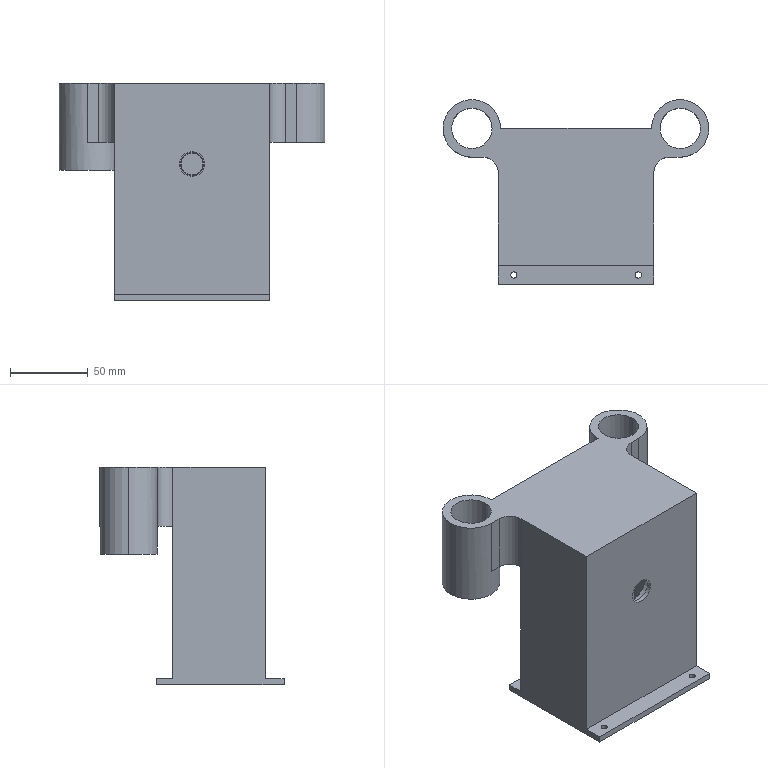Part | SolidWorks | features ICE 7, RevCut 2, Extrusion 1 | 1 solid | 68 faces | box 171 x 118.5 x 140 mm | volume 515598 mm3 | cylinder 37 | plane 31 | commonest cylinder face diameters 4 x8 15 x6 13.4 x4 26 x4 28 x4 37 x3